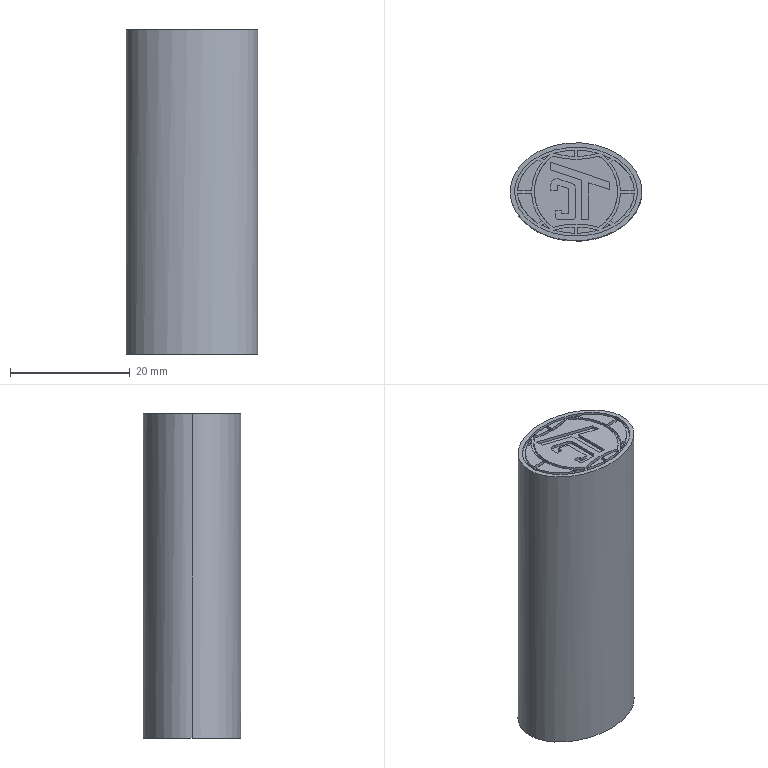Part | STEP file | LOGO LOM | 1 solid | 102 faces | box 22 x 16.4 x 54.3 mm | volume 14617 mm3 | plane 46 | spline 26 | cylinder 26 | cone 4 | commonest cylinder face diameters 26.92 x6 25.92 x4 29.02 x4 30.02 x4 0.4 x2 1.36 x2